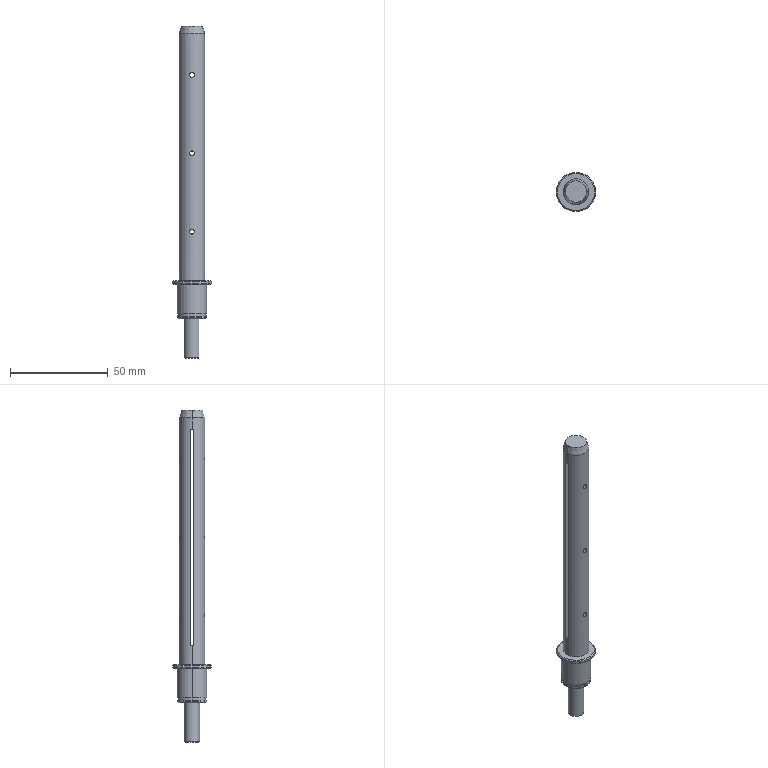Part | STEP file | 11-FG-B06011 | 1 solid | 45 faces | box 20 x 20 x 169.5 mm | volume 19381 mm3 | cylinder 23 | plane 12 | cone 10 | commonest cylinder face diameters 2.5 x12 15 x4 13 x2 14.3 x2 20 x2 8 x1